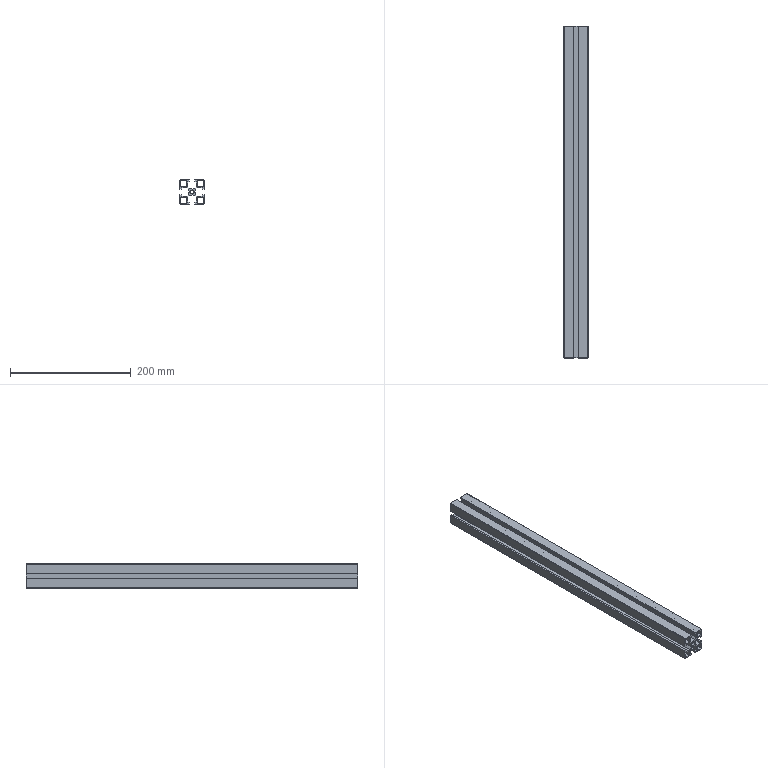Part | STEP file | 1 solid | 83 faces | box 40 x 550 x 40 mm | volume 261689 mm3 | plane 62 | cylinder 21 | commonest cylinder face diameters 1 x20 6.8 x1